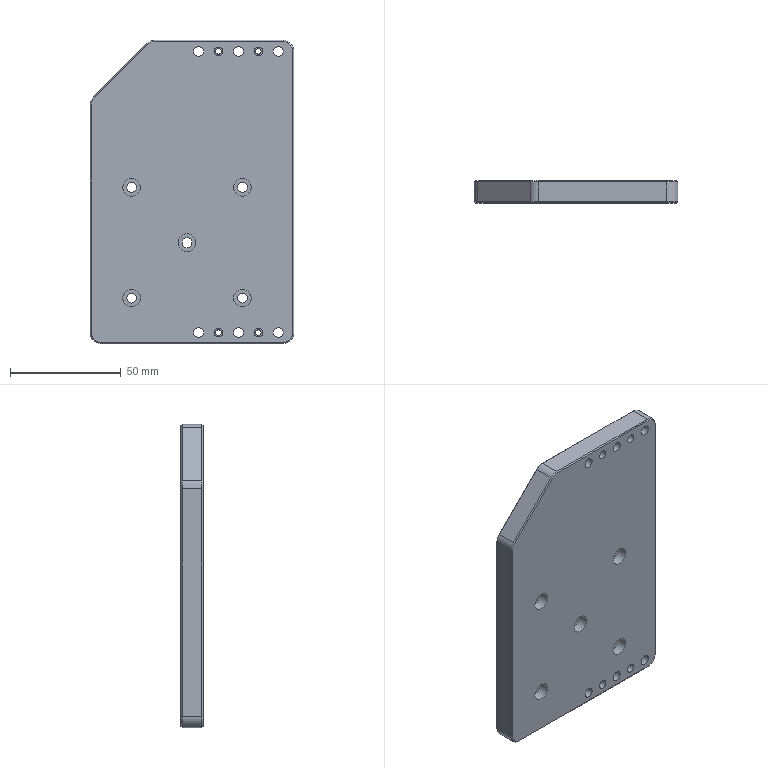CAM job | NX | 3+2 milling, drilling | part box 92 x 10 x 137 mm | stock box 95 x 12 x 142 mm
Tools:
number,name,description,diameter,corner_radius,flute_length,length,flutes
17,D2,平底铣刀-粗,2.0,0.0,50.0,75.0,2
4,D4,平底铣刀-粗,4.0,0.0,25.0,75.0,2
9,D10,平底铣刀-粗,10.0,0.0,35.0,75.0,2
18,D2-J,平底铣刀-精,2.0,0.0,50.0,75.0,2
10,D10-J,平底铣刀-精,10.0,0.0,35.0,75.0,2
1,D80R0.8飞刀,圆鼻刀-粗,80.0,0.8,50.0,75.0,2
1,D80R0.8飞刀-J,圆鼻刀-精,80.0,0.8,50.0,75.0,2
2,D6倒角刀,倒角刀,6.0,0.0,3.0,25.0,2
12,ZT2.5,钻头,2.5,0.0,35.0,50.0,2
11,ZT4.5,钻头,4.5,0.0,35.0,50.0,2
Operations:
program,operation,operation_type,tool,method,geometry_group,spindle_rpm,surface_speed,feed_per_tooth,feed_cut,feed_plunge,cut_length_mm,path_length_mm,cut_time_min,machine_time_min
B,底壁铣飞面开粗_COPY,VolumeBased25DMillingOperation,D80R0.8飞刀,分层开粗-切深K-步距G,W-B,2800.0,703.696,0.5357,3000.0,100.0,1969.852,2114.739,0.6566,0.6711
B,底壁铣飞面精光_COPY,VolumeBased25DMillingOperation,D80R0.8飞刀-J,侧刃精光-切深K-步距G,W-B,4000.0,1005.28,0.125,1000.0,100.0,491.884,527.884,0.4919,0.4955
B,铣沉头_1,CylinderMilling,D4,METHOD,W-B,6000.0,75.398,0.15,1800.0,100.0,1128.193,1592.993,0.6268,0.6733
B,铣孔_1,CylinderMilling,D4,METHOD,W-B,6000.0,75.398,0.05,600.0,100.0,105.106,599.306,0.1752,0.2246
B,钻倒角_2,Operation,D6倒角刀,METHOD,W-B,7000.0,131.947,0.0357,500.0,0.0,19.0,250.532,0.038,0.0612
B,钻倒角_3,Operation,D6倒角刀,METHOD,W-B,7000.0,131.947,0.0357,500.0,0.0,27.25,277.645,0.0545,0.0795
B,铣倒角_3,PlanarMilling,D6倒角刀,METHOD,W-B,7000.0,131.947,0.0429,600.0,100.0,122.676,579.694,0.2045,0.2502
B,底壁铣倒角_COPY_1,VolumeBased25DMillingOperation,D6倒角刀,爬面_倒角-切深0-步距G,W-B,6500.0,122.519,0.1154,1500.0,100.0,446.694,486.094,0.2978,0.3017
A,顶面,FaceMilling,D80R0.8飞刀,侧刃精光-切深K-步距G,W-A,5000.0,1256.637,0.1,1000.0,100.0,751.0,787.0,0.751,0.7546
A,型腔铣开粗-中_COPY,CavityMilling,D10,分层开粗-切深K-步距G,W-A,8000.0,251.32,0.25,4000.0,100.0,12107.856,12266.071,3.027,3.045
A,打点-深0.8,Operation,D6倒角刀,NONE,W-A,8000.0,150.796,0.0312,500.0,90.0,27.0,421.312,0.054,0.0934
A,通孔-精孔4.0预钻,Operation,ZT2.5,NONE,W-A,3000.0,36.757,0.0417,250.0,90.0,59.004,324.068,0.236,0.2625
A,通孔-5-6,Operation,ZT4.5,NONE,W-A,3000.0,42.411,0.0417,250.0,90.0,84.0,412.115,0.336,0.3688
A,沉头孔-钻孔0段,Operation,ZT4.5,NONE,W-A,2800.0,39.584,0.0357,200.0,90.0,71.76,358.278,0.3588,0.3875
A,铣孔开粗D4_1,CylinderMilling,D4,NONE,W-A,8000.0,100.531,0.075,1200.0,100.0,1064.784,1469.639,0.8873,0.9278
A,铣孔精光D4_1,CylinderMilling,D4,精光步距切深关,W-A,8000.0,100.531,0.0312,500.0,100.0,160.231,565.086,0.3205,0.3609
A,铣孔开粗D2_1,CylinderMilling,D2,NONE,W-A,8000.0,50.266,0.0375,600.0,100.0,780.044,1124.244,1.3,1.335
A,钻倒角_1,Operation,D6倒角刀,METHOD,W-A,8000.0,150.796,0.0312,500.0,0.0,21.2,254.932,0.0424,0.0658
A,铣倒角_1,PlanarMilling,D6倒角刀,METHOD,W-A,8000.0,150.796,0.0312,500.0,100.0,104.118,549.123,0.2082,0.2527
A,铣倒角_2,PlanarMilling,D6倒角刀,NONE,W-A,8000.0,150.796,0.0312,500.0,100.0,169.839,522.977,0.3397,0.375
A,底壁铣倒角_COPY,VolumeBased25DMillingOperation,D6倒角刀,爬面_倒角-切深0-步距G,W-A,6500.0,122.519,0.1154,1500.0,100.0,446.779,486.179,0.2979,0.3018
A,铣孔精光D2_1,CylinderMilling,D2-J,精光步距切深关,W-A,8000.0,50.266,0.0125,200.0,100.0,201.498,545.698,1.008,1.042
A,外形半精_2,VolumeBased25DMillingOperation,D10-J,METHOD,W-A,8000.0,251.327,0.0625,1000.0,100.0,471.728,530.928,0.4717,0.4776